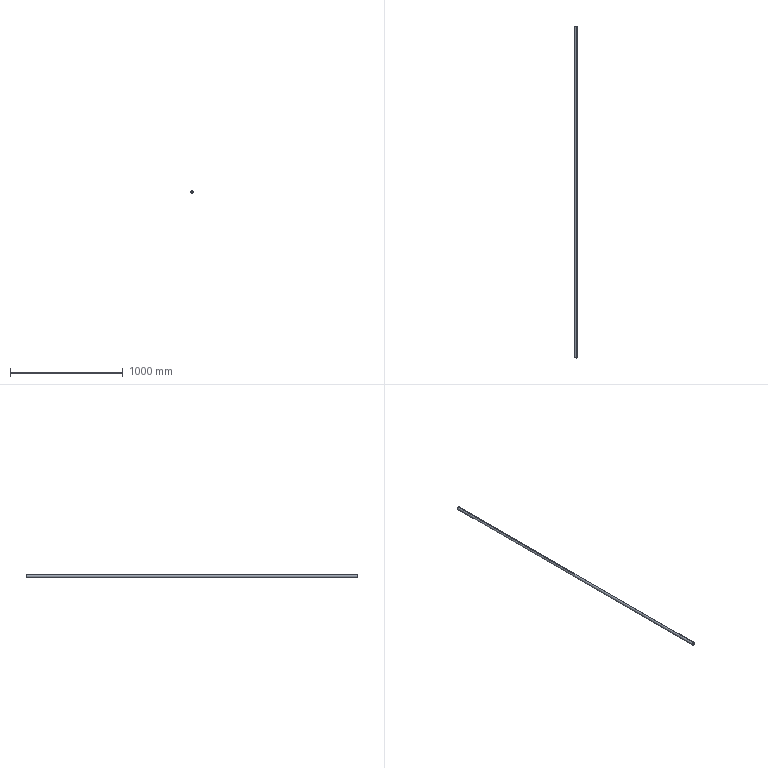Part | STEP file | PN_0039_Default<As Machined> | 1 solid | 6 faces | box 25.4 x 2940 x 25.4 mm | volume 584472 mm3 | cylinder 4 | plane 2 | commonest cylinder face diameters 19.8 x2 25.4 x2
STEP:
#1=CARTESIAN_POINT('',(0.,2940.,-9.9));
#2=VERTEX_POINT('',#1);
#3=CARTESIAN_POINT('',(0.,2940.,9.9));
#4=VERTEX_POINT('',#3);
#5=CARTESIAN_POINT('',(0.,2940.,0.));
#6=DIRECTION('',(0.,-1.,0.));
#7=AXIS2_PLACEMENT_3D('',#5,#6,$);
#8=CIRCLE('',#7,9.9);
#9=EDGE_CURVE('',#2,#4,#8,.F.);
#10=ORIENTED_EDGE('',*,*,#9,.T.);
#11=CARTESIAN_POINT('',(0.,0.,9.9));
#12=VERTEX_POINT('',#11);
#13=CARTESIAN_POINT('',(0.,2940.,9.9));
#14=DIRECTION('',(0.,-1.,0.));
#15=VECTOR('',#14,1.);
#16=LINE('',#13,#15);
#17=EDGE_CURVE('',#4,#12,#16,.T.);
#18=ORIENTED_EDGE('',*,*,#17,.T.);
#19=CARTESIAN_POINT('',(0.,0.,-9.9));
#20=VERTEX_POINT('',#19);
#21=CARTESIAN_POINT('',(0.,0.,0.));
#22=DIRECTION('',(0.,-1.,0.));
#23=AXIS2_PLACEMENT_3D('',#21,#22,$);
#24=CIRCLE('',#23,9.9);
#25=EDGE_CURVE('',#20,#12,#24,.F.);
#26=ORIENTED_EDGE('',*,*,#25,.F.);
#27=CARTESIAN_POINT('',(0.,2940.,-9.9));
#28=DIRECTION('',(0.,-1.,0.));
#29=VECTOR('',#28,1.);
#30=LINE('',#27,#29);
#31=EDGE_CURVE('',#2,#20,#30,.T.);
#32=ORIENTED_EDGE('',*,*,#31,.F.);
#33=EDGE_LOOP('',(#10,#18,#26,#32));
#34=FACE_OUTER_BOUND('',#33,.T.);
#35=CARTESIAN_POINT('',(0.,2940.,0.));
#36=DIRECTION('',(0.,-1.,0.));
#37=DIRECTION('',(0.,0.,1.));
#38=AXIS2_PLACEMENT_3D('',#35,#36,#37);
#39=CYLINDRICAL_SURFACE('',#38,9.9);
#40=ADVANCED_FACE('',(#34),#39,.F.);
#41=CARTESIAN_POINT('',(0.,2940.,-12.7));
#42=VERTEX_POINT('',#41);
#43=CARTESIAN_POINT('',(0.,2940.,12.7));
#44=VERTEX_POINT('',#43);
#45=CARTESIAN_POINT('',(0.,2940.,0.));
#46=DIRECTION('',(0.,1.,0.));
#47=AXIS2_PLACEMENT_3D('',#45,#46,$);
#48=CIRCLE('',#47,12.7);
#49=EDGE_CURVE('',#42,#44,#48,.T.);
#50=ORIENTED_EDGE('',*,*,#49,.T.);
#51=CARTESIAN_POINT('',(0.,2940.,0.));
#52=DIRECTION('',(0.,1.,0.));
#53=AXIS2_PLACEMENT_3D('',#51,#52,$);
#54=CIRCLE('',#53,12.7);
#55=EDGE_CURVE('',#44,#42,#54,.T.);
#56=ORIENTED_EDGE('',*,*,#55,.T.);
#57=EDGE_LOOP('',(#50,#56));
#58=FACE_OUTER_BOUND('',#57,.T.);
#59=ORIENTED_EDGE('',*,*,#9,.F.);
#60=CARTESIAN_POINT('',(0.,2940.,0.));
#61=DIRECTION('',(0.,1.,0.));
#62=AXIS2_PLACEMENT_3D('',#60,#61,$);
#63=CIRCLE('',#62,9.9);
#64=EDGE_CURVE('',#4,#2,#63,.T.);
#65=ORIENTED_EDGE('',*,*,#64,.F.);
#66=EDGE_LOOP('',(#59,#65));
#67=FACE_BOUND('',#66,.T.);
#68=CARTESIAN_POINT('',(0.,2940.,0.));
#69=DIRECTION('',(0.,1.,0.));
#70=DIRECTION('',(0.,0.,1.));
#71=AXIS2_PLACEMENT_3D('',#68,#69,#70);
#72=PLANE('',#71);
#73=ADVANCED_FACE('',(#58,#67),#72,.T.);
#74=ORIENTED_EDGE('',*,*,#17,.F.);
#75=ORIENTED_EDGE('',*,*,#64,.T.);
#76=ORIENTED_EDGE('',*,*,#31,.T.);
#77=CARTESIAN_POINT('',(0.,0.,0.));
#78=DIRECTION('',(0.,-1.,0.));
#79=AXIS2_PLACEMENT_3D('',#77,#78,$);
#80=CIRCLE('',#79,9.9);
#81=EDGE_CURVE('',#12,#20,#80,.F.);
#82=ORIENTED_EDGE('',*,*,#81,.F.);
#83=EDGE_LOOP('',(#74,#75,#76,#82));
#84=FACE_OUTER_BOUND('',#83,.T.);
#85=CARTESIAN_POINT('',(0.,2940.,0.));
#86=DIRECTION('',(0.,-1.,0.));
#87=DIRECTION('',(0.,0.,-1.));
#88=AXIS2_PLACEMENT_3D('',#85,#86,#87);
#89=CYLINDRICAL_SURFACE('',#88,9.9);
#90=ADVANCED_FACE('',(#84),#89,.F.);
#91=CARTESIAN_POINT('',(0.,0.,-12.7));
#92=VERTEX_POINT('',#91);
#93=CARTESIAN_POINT('',(0.,0.,12.7));
#94=VERTEX_POINT('',#93);
#95=CARTESIAN_POINT('',(0.,0.,0.));
#96=DIRECTION('',(0.,1.,0.));
#97=AXIS2_PLACEMENT_3D('',#95,#96,$);
#98=CIRCLE('',#97,12.7);
#99=EDGE_CURVE('',#92,#94,#98,.T.);
#100=ORIENTED_EDGE('',*,*,#99,.F.);
#101=CARTESIAN_POINT('',(0.,0.,0.));
#102=DIRECTION('',(0.,1.,0.));
#103=AXIS2_PLACEMENT_3D('',#101,#102,$);
#104=CIRCLE('',#103,12.7);
#105=EDGE_CURVE('',#94,#92,#104,.T.);
#106=ORIENTED_EDGE('',*,*,#105,.F.);
#107=EDGE_LOOP('',(#100,#106));
#108=FACE_OUTER_BOUND('',#107,.T.);
#109=ORIENTED_EDGE('',*,*,#25,.T.);
#110=ORIENTED_EDGE('',*,*,#81,.T.);
#111=EDGE_LOOP('',(#109,#110));
#112=FACE_BOUND('',#111,.T.);
#113=CARTESIAN_POINT('',(0.,0.,0.));
#114=DIRECTION('',(0.,1.,0.));
#115=DIRECTION('',(0.,0.,1.));
#116=AXIS2_PLACEMENT_3D('',#113,#114,#115);
#117=PLANE('',#116);
#118=ADVANCED_FACE('',(#108,#112),#117,.F.);
#119=CARTESIAN_POINT('',(0.,2940.,12.7));
#120=DIRECTION('',(0.,-1.,0.));
#121=VECTOR('',#120,1.);
#122=LINE('',#119,#121);
#123=EDGE_CURVE('',#44,#94,#122,.T.);
#124=ORIENTED_EDGE('',*,*,#123,.F.);
#125=ORIENTED_EDGE('',*,*,#49,.F.);
#126=CARTESIAN_POINT('',(0.,2940.,-12.7));
#127=DIRECTION('',(0.,-1.,0.));
#128=VECTOR('',#127,1.);
#129=LINE('',#126,#128);
#130=EDGE_CURVE('',#42,#92,#129,.T.);
#131=ORIENTED_EDGE('',*,*,#130,.T.);
#132=ORIENTED_EDGE('',*,*,#99,.T.);
#133=EDGE_LOOP('',(#124,#125,#131,#132));
#134=FACE_OUTER_BOUND('',#133,.T.);
#135=CARTESIAN_POINT('',(0.,2940.,0.));
#136=DIRECTION('',(0.,-1.,0.));
#137=DIRECTION('',(0.,0.,1.));
#138=AXIS2_PLACEMENT_3D('',#135,#136,#137);
#139=CYLINDRICAL_SURFACE('',#138,12.7);
#140=ADVANCED_FACE('',(#134),#139,.T.);
#141=ORIENTED_EDGE('',*,*,#55,.F.);
#142=ORIENTED_EDGE('',*,*,#123,.T.);
#143=ORIENTED_EDGE('',*,*,#105,.T.);
#144=ORIENTED_EDGE('',*,*,#130,.F.);
#145=EDGE_LOOP('',(#141,#142,#143,#144));
#146=FACE_OUTER_BOUND('',#145,.T.);
#147=CARTESIAN_POINT('',(0.,2940.,0.));
#148=DIRECTION('',(0.,-1.,0.));
#149=DIRECTION('',(0.,0.,-1.));
#150=AXIS2_PLACEMENT_3D('',#147,#148,#149);
#151=CYLINDRICAL_SURFACE('',#150,12.7);
#152=ADVANCED_FACE('',(#146),#151,.T.);
#153=CLOSED_SHELL('',(#40,#73,#90,#118,#140,#152));
#154=MANIFOLD_SOLID_BREP('',#153);
#155=(LENGTH_UNIT()NAMED_UNIT(*)SI_UNIT(.MILLI.,.METRE.));
#156=UNCERTAINTY_MEASURE_WITH_UNIT(LENGTH_MEASURE(0.005),#155,'','');
#157=(NAMED_UNIT(*)PLANE_ANGLE_UNIT()SI_UNIT($,.RADIAN.));
#158=(NAMED_UNIT(*)SI_UNIT($,.STERADIAN.)SOLID_ANGLE_UNIT());
#159=(GEOMETRIC_REPRESENTATION_CONTEXT(3)GLOBAL_UNCERTAINTY_ASSIGNED_CONTEXT((#156))GLOBAL_UNIT_ASSIGNED_CONTEXT((#155,#157,#158))REPRESENTATION_CONTEXT('',''));
#160=ADVANCED_BREP_SHAPE_REPRESENTATION('',(#154),#159);